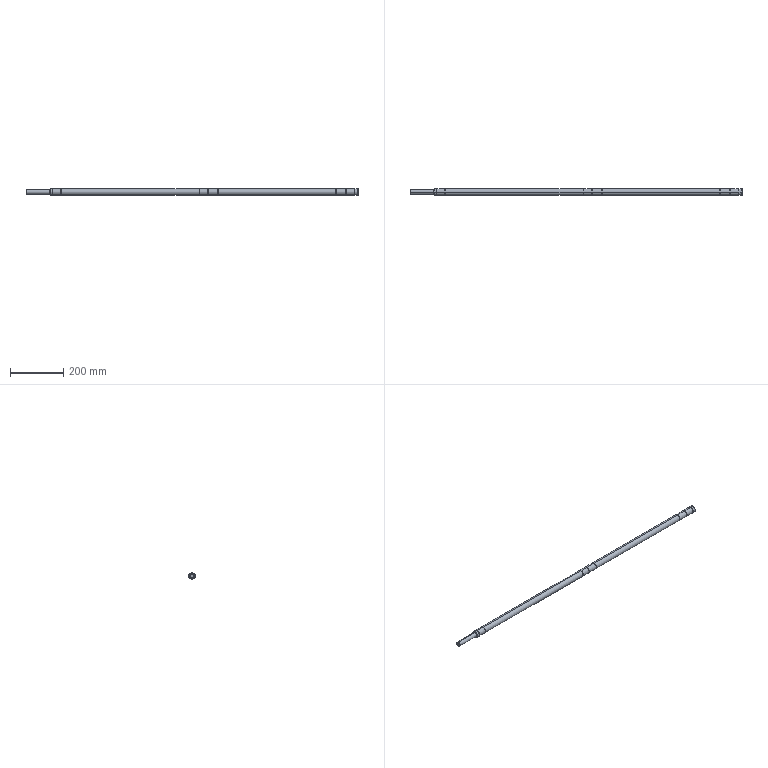Part | SolidWorks | features ICE 6, Chamfer 2, RevCut 2, Extrusion 1, Fillet 1, HoleWzd 1, LPattern 1 | 1 solid | 81 faces | box 1244 x 25 x 25 mm | volume 582706 mm3 | cylinder 44 | plane 31 | cone 4 | torus 2 | commonest cylinder face diameters 25 x18 24 x16 8 x6 5 x2 17 x2